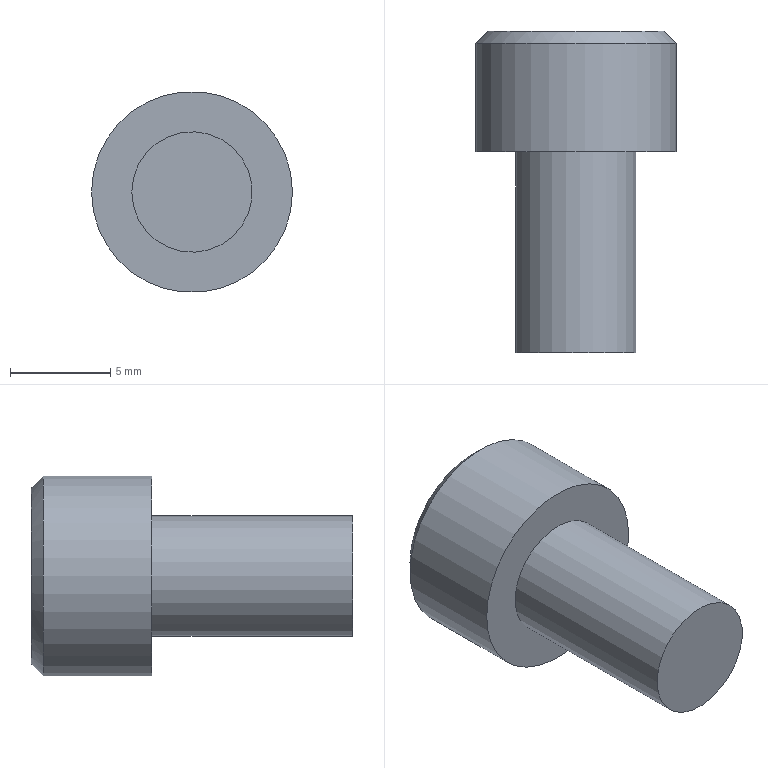Part | NX | features 5003_326_CB6-10 2 | 1 solid | 19 faces | box 10 x 16 x 10 mm | volume 673.77 mm3 | plane 15 | cylinder 2 | cone 2 | commonest cylinder face diameters 6 x1 10 x1
STEP:
#1=CARTESIAN_POINT('',(170.225,6.,-39.5));
#2=VERTEX_POINT('',#1);
#3=CARTESIAN_POINT('',(165.825,6.,-39.5));
#4=DIRECTION('',(0.,-1.,0.));
#5=DIRECTION('',(1.,0.,0.));
#6=AXIS2_PLACEMENT_3D('',#3,#4,#5);
#7=CIRCLE('',#6,4.4);
#8=EDGE_CURVE('',#2,#2,#7,.F.);
#9=ORIENTED_EDGE('',*,*,#8,.T.);
#10=EDGE_LOOP('',(#9));
#11=FACE_BOUND('',#10,.T.);
#12=CARTESIAN_POINT('',(165.825,6.,-42.387));
#13=VERTEX_POINT('',#12);
#14=CARTESIAN_POINT('',(163.325,6.,-40.943));
#15=VERTEX_POINT('',#14);
#16=CARTESIAN_POINT('',(165.825,6.,-42.387));
#17=DIRECTION('',(-0.866,0.,0.5));
#18=VECTOR('',#17,1000.);
#19=LINE('',#16,#18);
#20=EDGE_CURVE('',#13,#15,#19,.T.);
#21=ORIENTED_EDGE('',*,*,#20,.F.);
#22=CARTESIAN_POINT('',(168.325,6.,-40.943));
#23=VERTEX_POINT('',#22);
#24=CARTESIAN_POINT('',(168.325,6.,-40.943));
#25=DIRECTION('',(-0.866,0.,-0.5));
#26=VECTOR('',#25,1000.);
#27=LINE('',#24,#26);
#28=EDGE_CURVE('',#23,#13,#27,.T.);
#29=ORIENTED_EDGE('',*,*,#28,.F.);
#30=CARTESIAN_POINT('',(168.325,6.,-38.057));
#31=VERTEX_POINT('',#30);
#32=CARTESIAN_POINT('',(168.325,6.,-38.057));
#33=DIRECTION('',(0.,0.,-1.));
#34=VECTOR('',#33,1000.);
#35=LINE('',#32,#34);
#36=EDGE_CURVE('',#31,#23,#35,.T.);
#37=ORIENTED_EDGE('',*,*,#36,.F.);
#38=CARTESIAN_POINT('',(165.825,6.,-36.613));
#39=VERTEX_POINT('',#38);
#40=CARTESIAN_POINT('',(165.825,6.,-36.613));
#41=DIRECTION('',(0.866,0.,-0.5));
#42=VECTOR('',#41,1000.);
#43=LINE('',#40,#42);
#44=EDGE_CURVE('',#39,#31,#43,.T.);
#45=ORIENTED_EDGE('',*,*,#44,.F.);
#46=CARTESIAN_POINT('',(163.325,6.,-38.057));
#47=VERTEX_POINT('',#46);
#48=CARTESIAN_POINT('',(163.325,6.,-38.057));
#49=DIRECTION('',(0.866,0.,0.5));
#50=VECTOR('',#49,1000.);
#51=LINE('',#48,#50);
#52=EDGE_CURVE('',#47,#39,#51,.T.);
#53=ORIENTED_EDGE('',*,*,#52,.F.);
#54=CARTESIAN_POINT('',(163.325,6.,-40.943));
#55=DIRECTION('',(0.,0.,1.));
#56=VECTOR('',#55,1000.);
#57=LINE('',#54,#56);
#58=EDGE_CURVE('',#15,#47,#57,.T.);
#59=ORIENTED_EDGE('',*,*,#58,.F.);
#60=EDGE_LOOP('',(#21,#29,#37,#45,#53,#59));
#61=FACE_BOUND('',#60,.T.);
#62=CARTESIAN_POINT('',(165.825,6.,-34.5));
#63=DIRECTION('',(0.,-1.,0.));
#64=DIRECTION('',(1.,0.,0.));
#65=AXIS2_PLACEMENT_3D('',#62,#63,#64);
#66=PLANE('',#65);
#67=ADVANCED_FACE('',(#11,#61),#66,.F.);
#68=CARTESIAN_POINT('',(162.825,-10.,-39.5));
#69=VERTEX_POINT('',#68);
#70=CARTESIAN_POINT('',(165.825,-10.,-39.5));
#71=DIRECTION('',(0.,1.,0.));
#72=DIRECTION('',(-1.,0.,0.));
#73=AXIS2_PLACEMENT_3D('',#70,#71,#72);
#74=CIRCLE('',#73,3.);
#75=EDGE_CURVE('',#69,#69,#74,.T.);
#76=ORIENTED_EDGE('',*,*,#75,.F.);
#77=EDGE_LOOP('',(#76));
#78=FACE_BOUND('',#77,.T.);
#79=CARTESIAN_POINT('',(165.825,-10.,-39.5));
#80=DIRECTION('',(0.,1.,0.));
#81=DIRECTION('',(-1.,0.,0.));
#82=AXIS2_PLACEMENT_3D('',#79,#80,#81);
#83=PLANE('',#82);
#84=ADVANCED_FACE('',(#78),#83,.F.);
#85=CARTESIAN_POINT('',(162.825,0.,-39.5));
#86=VERTEX_POINT('',#85);
#87=CARTESIAN_POINT('',(165.825,0.,-39.5));
#88=DIRECTION('',(0.,1.,0.));
#89=DIRECTION('',(-1.,0.,0.));
#90=AXIS2_PLACEMENT_3D('',#87,#88,#89);
#91=CIRCLE('',#90,3.);
#92=EDGE_CURVE('',#86,#86,#91,.T.);
#93=ORIENTED_EDGE('',*,*,#92,.F.);
#94=EDGE_LOOP('',(#93));
#95=FACE_BOUND('',#94,.T.);
#96=ORIENTED_EDGE('',*,*,#75,.T.);
#97=EDGE_LOOP('',(#96));
#98=FACE_BOUND('',#97,.T.);
#99=CARTESIAN_POINT('',(165.825,6.,-39.5));
#100=DIRECTION('',(0.,1.,0.));
#101=DIRECTION('',(-1.,0.,0.));
#102=AXIS2_PLACEMENT_3D('',#99,#100,#101);
#103=CYLINDRICAL_SURFACE('',#102,3.);
#104=ADVANCED_FACE('',(#95,#98),#103,.T.);
#105=CARTESIAN_POINT('',(160.825,0.,-39.5));
#106=VERTEX_POINT('',#105);
#107=CARTESIAN_POINT('',(165.825,0.,-39.5));
#108=DIRECTION('',(0.,1.,0.));
#109=DIRECTION('',(-1.,0.,0.));
#110=AXIS2_PLACEMENT_3D('',#107,#108,#109);
#111=CIRCLE('',#110,5.);
#112=EDGE_CURVE('',#106,#106,#111,.T.);
#113=ORIENTED_EDGE('',*,*,#112,.F.);
#114=EDGE_LOOP('',(#113));
#115=FACE_BOUND('',#114,.T.);
#116=ORIENTED_EDGE('',*,*,#92,.T.);
#117=EDGE_LOOP('',(#116));
#118=FACE_BOUND('',#117,.T.);
#119=CARTESIAN_POINT('',(165.825,0.,-36.5));
#120=DIRECTION('',(0.,1.,0.));
#121=DIRECTION('',(-1.,0.,0.));
#122=AXIS2_PLACEMENT_3D('',#119,#120,#121);
#123=PLANE('',#122);
#124=ADVANCED_FACE('',(#115,#118),#123,.F.);
#125=CARTESIAN_POINT('',(170.825,5.4,-39.5));
#126=VERTEX_POINT('',#125);
#127=CARTESIAN_POINT('',(165.825,5.4,-39.5));
#128=DIRECTION('',(0.,-1.,0.));
#129=DIRECTION('',(1.,0.,0.));
#130=AXIS2_PLACEMENT_3D('',#127,#128,#129);
#131=CIRCLE('',#130,5.);
#132=EDGE_CURVE('',#126,#126,#131,.T.);
#133=ORIENTED_EDGE('',*,*,#132,.T.);
#134=EDGE_LOOP('',(#133));
#135=FACE_BOUND('',#134,.T.);
#136=ORIENTED_EDGE('',*,*,#112,.T.);
#137=EDGE_LOOP('',(#136));
#138=FACE_BOUND('',#137,.T.);
#139=CARTESIAN_POINT('',(165.825,6.,-39.5));
#140=DIRECTION('',(0.,1.,0.));
#141=DIRECTION('',(-1.,0.,0.));
#142=AXIS2_PLACEMENT_3D('',#139,#140,#141);
#143=CYLINDRICAL_SURFACE('',#142,5.);
#144=ADVANCED_FACE('',(#135,#138),#143,.T.);
#145=ORIENTED_EDGE('',*,*,#132,.F.);
#146=EDGE_LOOP('',(#145));
#147=FACE_BOUND('',#146,.T.);
#148=ORIENTED_EDGE('',*,*,#8,.F.);
#149=EDGE_LOOP('',(#148));
#150=FACE_BOUND('',#149,.T.);
#151=CARTESIAN_POINT('',(165.825,6.,-39.5));
#152=DIRECTION('',(0.,-1.,0.));
#153=DIRECTION('',(1.,0.,0.));
#154=AXIS2_PLACEMENT_3D('',#151,#152,#153);
#155=CONICAL_SURFACE('',#154,4.4,0.7854);
#156=ADVANCED_FACE('',(#147,#150),#155,.T.);
#157=CARTESIAN_POINT('',(168.325,3.,-40.943));
#158=VERTEX_POINT('',#157);
#159=CARTESIAN_POINT('',(167.075,3.,-41.665));
#160=VERTEX_POINT('',#159);
#161=CARTESIAN_POINT('',(168.325,3.,-40.943));
#162=DIRECTION('',(-0.866,0.,-0.5));
#163=VECTOR('',#162,1000.);
#164=LINE('',#161,#163);
#165=EDGE_CURVE('',#158,#160,#164,.T.);
#166=ORIENTED_EDGE('',*,*,#165,.F.);
#167=CARTESIAN_POINT('',(168.325,3.,-40.943));
#168=DIRECTION('',(0.,1.,0.));
#169=VECTOR('',#168,1000.);
#170=LINE('',#167,#169);
#171=EDGE_CURVE('',#158,#23,#170,.T.);
#172=ORIENTED_EDGE('',*,*,#171,.T.);
#173=ORIENTED_EDGE('',*,*,#28,.T.);
#174=CARTESIAN_POINT('',(165.825,3.,-42.387));
#175=VERTEX_POINT('',#174);
#176=CARTESIAN_POINT('',(165.825,3.,-42.387));
#177=DIRECTION('',(0.,1.,0.));
#178=VECTOR('',#177,1000.);
#179=LINE('',#176,#178);
#180=EDGE_CURVE('',#175,#13,#179,.T.);
#181=ORIENTED_EDGE('',*,*,#180,.F.);
#182=CARTESIAN_POINT('',(168.325,3.,-40.943));
#183=DIRECTION('',(-0.866,0.,-0.5));
#184=VECTOR('',#183,1000.);
#185=LINE('',#182,#184);
#186=EDGE_CURVE('',#160,#175,#185,.T.);
#187=ORIENTED_EDGE('',*,*,#186,.F.);
#188=EDGE_LOOP('',(#166,#172,#173,#181,#187));
#189=FACE_BOUND('',#188,.T.);
#190=CARTESIAN_POINT('',(168.325,3.,-40.943));
#191=DIRECTION('',(0.5,0.,-0.866));
#192=DIRECTION('',(0.866,0.,0.5));
#193=AXIS2_PLACEMENT_3D('',#190,#191,#192);
#194=PLANE('',#193);
#195=ADVANCED_FACE('',(#189),#194,.F.);
#196=CARTESIAN_POINT('',(168.325,3.,-38.057));
#197=VERTEX_POINT('',#196);
#198=CARTESIAN_POINT('',(168.325,3.,-39.5));
#199=VERTEX_POINT('',#198);
#200=CARTESIAN_POINT('',(168.325,3.,-38.057));
#201=DIRECTION('',(0.,0.,-1.));
#202=VECTOR('',#201,1000.);
#203=LINE('',#200,#202);
#204=EDGE_CURVE('',#197,#199,#203,.T.);
#205=ORIENTED_EDGE('',*,*,#204,.F.);
#206=CARTESIAN_POINT('',(168.325,3.,-38.057));
#207=DIRECTION('',(0.,1.,0.));
#208=VECTOR('',#207,1000.);
#209=LINE('',#206,#208);
#210=EDGE_CURVE('',#197,#31,#209,.T.);
#211=ORIENTED_EDGE('',*,*,#210,.T.);
#212=ORIENTED_EDGE('',*,*,#36,.T.);
#213=ORIENTED_EDGE('',*,*,#171,.F.);
#214=CARTESIAN_POINT('',(168.325,3.,-38.057));
#215=DIRECTION('',(0.,0.,-1.));
#216=VECTOR('',#215,1000.);
#217=LINE('',#214,#216);
#218=EDGE_CURVE('',#199,#158,#217,.T.);
#219=ORIENTED_EDGE('',*,*,#218,.F.);
#220=EDGE_LOOP('',(#205,#211,#212,#213,#219));
#221=FACE_BOUND('',#220,.T.);
#222=CARTESIAN_POINT('',(168.325,3.,-38.057));
#223=DIRECTION('',(1.,0.,0.));
#224=DIRECTION('',(0.,0.,1.));
#225=AXIS2_PLACEMENT_3D('',#222,#223,#224);
#226=PLANE('',#225);
#227=ADVANCED_FACE('',(#221),#226,.F.);
#228=CARTESIAN_POINT('',(165.825,3.,-36.613));
#229=VERTEX_POINT('',#228);
#230=CARTESIAN_POINT('',(167.075,3.,-37.335));
#231=VERTEX_POINT('',#230);
#232=CARTESIAN_POINT('',(165.825,3.,-36.613));
#233=DIRECTION('',(0.866,0.,-0.5));
#234=VECTOR('',#233,1000.);
#235=LINE('',#232,#234);
#236=EDGE_CURVE('',#229,#231,#235,.T.);
#237=ORIENTED_EDGE('',*,*,#236,.F.);
#238=CARTESIAN_POINT('',(165.825,3.,-36.613));
#239=DIRECTION('',(0.,1.,0.));
#240=VECTOR('',#239,1000.);
#241=LINE('',#238,#240);
#242=EDGE_CURVE('',#229,#39,#241,.T.);
#243=ORIENTED_EDGE('',*,*,#242,.T.);
#244=ORIENTED_EDGE('',*,*,#44,.T.);
#245=ORIENTED_EDGE('',*,*,#210,.F.);
#246=CARTESIAN_POINT('',(165.825,3.,-36.613));
#247=DIRECTION('',(0.866,0.,-0.5));
#248=VECTOR('',#247,1000.);
#249=LINE('',#246,#248);
#250=EDGE_CURVE('',#231,#197,#249,.T.);
#251=ORIENTED_EDGE('',*,*,#250,.F.);
#252=EDGE_LOOP('',(#237,#243,#244,#245,#251));
#253=FACE_BOUND('',#252,.T.);
#254=CARTESIAN_POINT('',(165.825,3.,-36.613));
#255=DIRECTION('',(0.5,0.,0.866));
#256=DIRECTION('',(-0.866,0.,0.5));
#257=AXIS2_PLACEMENT_3D('',#254,#255,#256);
#258=PLANE('',#257);
#259=ADVANCED_FACE('',(#253),#258,.F.);
#260=CARTESIAN_POINT('',(163.325,3.,-38.057));
#261=VERTEX_POINT('',#260);
#262=CARTESIAN_POINT('',(164.575,3.,-37.335));
#263=VERTEX_POINT('',#262);
#264=CARTESIAN_POINT('',(163.325,3.,-38.057));
#265=DIRECTION('',(0.866,0.,0.5));
#266=VECTOR('',#265,1000.);
#267=LINE('',#264,#266);
#268=EDGE_CURVE('',#261,#263,#267,.T.);
#269=ORIENTED_EDGE('',*,*,#268,.F.);
#270=CARTESIAN_POINT('',(163.325,3.,-38.057));
#271=DIRECTION('',(0.,1.,0.));
#272=VECTOR('',#271,1000.);
#273=LINE('',#270,#272);
#274=EDGE_CURVE('',#261,#47,#273,.T.);
#275=ORIENTED_EDGE('',*,*,#274,.T.);
#276=ORIENTED_EDGE('',*,*,#52,.T.);
#277=ORIENTED_EDGE('',*,*,#242,.F.);
#278=CARTESIAN_POINT('',(163.325,3.,-38.057));
#279=DIRECTION('',(0.866,0.,0.5));
#280=VECTOR('',#279,1000.);
#281=LINE('',#278,#280);
#282=EDGE_CURVE('',#263,#229,#281,.T.);
#283=ORIENTED_EDGE('',*,*,#282,.F.);
#284=EDGE_LOOP('',(#269,#275,#276,#277,#283));
#285=FACE_BOUND('',#284,.T.);
#286=CARTESIAN_POINT('',(163.325,3.,-38.057));
#287=DIRECTION('',(-0.5,0.,0.866));
#288=DIRECTION('',(-0.866,0.,-0.5));
#289=AXIS2_PLACEMENT_3D('',#286,#287,#288);
#290=PLANE('',#289);
#291=ADVANCED_FACE('',(#285),#290,.F.);
#292=CARTESIAN_POINT('',(163.325,3.,-40.943));
#293=VERTEX_POINT('',#292);
#294=CARTESIAN_POINT('',(163.325,3.,-39.5));
#295=VERTEX_POINT('',#294);
#296=CARTESIAN_POINT('',(163.325,3.,-40.943));
#297=DIRECTION('',(0.,0.,1.));
#298=VECTOR('',#297,1000.);
#299=LINE('',#296,#298);
#300=EDGE_CURVE('',#293,#295,#299,.T.);
#301=ORIENTED_EDGE('',*,*,#300,.F.);
#302=CARTESIAN_POINT('',(163.325,3.,-40.943));
#303=DIRECTION('',(0.,1.,0.));
#304=VECTOR('',#303,1000.);
#305=LINE('',#302,#304);
#306=EDGE_CURVE('',#293,#15,#305,.T.);
#307=ORIENTED_EDGE('',*,*,#306,.T.);
#308=ORIENTED_EDGE('',*,*,#58,.T.);
#309=ORIENTED_EDGE('',*,*,#274,.F.);
#310=CARTESIAN_POINT('',(163.325,3.,-40.943));
#311=DIRECTION('',(0.,0.,1.));
#312=VECTOR('',#311,1000.);
#313=LINE('',#310,#312);
#314=EDGE_CURVE('',#295,#261,#313,.T.);
#315=ORIENTED_EDGE('',*,*,#314,.F.);
#316=EDGE_LOOP('',(#301,#307,#308,#309,#315));
#317=FACE_BOUND('',#316,.T.);
#318=CARTESIAN_POINT('',(163.325,3.,-40.943));
#319=DIRECTION('',(-1.,0.,0.));
#320=DIRECTION('',(0.,-1.,0.));
#321=AXIS2_PLACEMENT_3D('',#318,#319,#320);
#322=PLANE('',#321);
#323=ADVANCED_FACE('',(#317),#322,.F.);
#324=CARTESIAN_POINT('',(164.575,3.,-41.665));
#325=VERTEX_POINT('',#324);
#326=CARTESIAN_POINT('',(165.825,3.,-42.387));
#327=DIRECTION('',(-0.866,0.,0.5));
#328=VECTOR('',#327,1000.);
#329=LINE('',#326,#328);
#330=EDGE_CURVE('',#175,#325,#329,.T.);
#331=ORIENTED_EDGE('',*,*,#330,.F.);
#332=ORIENTED_EDGE('',*,*,#180,.T.);
#333=ORIENTED_EDGE('',*,*,#20,.T.);
#334=ORIENTED_EDGE('',*,*,#306,.F.);
#335=CARTESIAN_POINT('',(165.825,3.,-42.387));
#336=DIRECTION('',(-0.866,0.,0.5));
#337=VECTOR('',#336,1000.);
#338=LINE('',#335,#337);
#339=EDGE_CURVE('',#325,#293,#338,.T.);
#340=ORIENTED_EDGE('',*,*,#339,.F.);
#341=EDGE_LOOP('',(#331,#332,#333,#334,#340));
#342=FACE_BOUND('',#341,.T.);
#343=CARTESIAN_POINT('',(165.825,3.,-42.387));
#344=DIRECTION('',(-0.5,0.,-0.866));
#345=DIRECTION('',(0.866,0.,-0.5));
#346=AXIS2_PLACEMENT_3D('',#343,#344,#345);
#347=PLANE('',#346);
#348=ADVANCED_FACE('',(#342),#347,.F.);
#349=ORIENTED_EDGE('',*,*,#314,.T.);
#350=ORIENTED_EDGE('',*,*,#268,.T.);
#351=CARTESIAN_POINT('',(165.825,3.,-39.5));
#352=DIRECTION('',(0.,1.,0.));
#353=DIRECTION('',(0.,0.,-1.));
#354=AXIS2_PLACEMENT_3D('',#351,#352,#353);
#355=CIRCLE('',#354,2.5);
#356=EDGE_CURVE('',#295,#263,#355,.T.);
#357=ORIENTED_EDGE('',*,*,#356,.F.);
#358=EDGE_LOOP('',(#349,#350,#357));
#359=FACE_BOUND('',#358,.T.);
#360=CARTESIAN_POINT('',(165.825,3.,-39.5));
#361=DIRECTION('',(0.,1.,0.));
#362=DIRECTION('',(-1.,0.,0.));
#363=AXIS2_PLACEMENT_3D('',#360,#361,#362);
#364=PLANE('',#363);
#365=ADVANCED_FACE('',(#359),#364,.T.);
#366=ORIENTED_EDGE('',*,*,#282,.T.);
#367=ORIENTED_EDGE('',*,*,#236,.T.);
#368=CARTESIAN_POINT('',(165.825,3.,-39.5));
#369=DIRECTION('',(0.,1.,0.));
#370=DIRECTION('',(0.,0.,-1.));
#371=AXIS2_PLACEMENT_3D('',#368,#369,#370);
#372=CIRCLE('',#371,2.5);
#373=EDGE_CURVE('',#263,#231,#372,.T.);
#374=ORIENTED_EDGE('',*,*,#373,.F.);
#375=EDGE_LOOP('',(#366,#367,#374));
#376=FACE_BOUND('',#375,.T.);
#377=CARTESIAN_POINT('',(165.825,3.,-39.5));
#378=DIRECTION('',(0.,1.,0.));
#379=DIRECTION('',(-1.,0.,0.));
#380=AXIS2_PLACEMENT_3D('',#377,#378,#379);
#381=PLANE('',#380);
#382=ADVANCED_FACE('',(#376),#381,.T.);
#383=ORIENTED_EDGE('',*,*,#250,.T.);
#384=ORIENTED_EDGE('',*,*,#204,.T.);
#385=CARTESIAN_POINT('',(165.825,3.,-39.5));
#386=DIRECTION('',(0.,1.,0.));
#387=DIRECTION('',(0.,0.,-1.));
#388=AXIS2_PLACEMENT_3D('',#385,#386,#387);
#389=CIRCLE('',#388,2.5);
#390=EDGE_CURVE('',#231,#199,#389,.T.);
#391=ORIENTED_EDGE('',*,*,#390,.F.);
#392=EDGE_LOOP('',(#383,#384,#391));
#393=FACE_BOUND('',#392,.T.);
#394=CARTESIAN_POINT('',(165.825,3.,-39.5));
#395=DIRECTION('',(0.,1.,0.));
#396=DIRECTION('',(-1.,0.,0.));
#397=AXIS2_PLACEMENT_3D('',#394,#395,#396);
#398=PLANE('',#397);
#399=ADVANCED_FACE('',(#393),#398,.T.);
#400=ORIENTED_EDGE('',*,*,#218,.T.);
#401=ORIENTED_EDGE('',*,*,#165,.T.);
#402=CARTESIAN_POINT('',(165.825,3.,-39.5));
#403=DIRECTION('',(0.,1.,0.));
#404=DIRECTION('',(0.,0.,-1.));
#405=AXIS2_PLACEMENT_3D('',#402,#403,#404);
#406=CIRCLE('',#405,2.5);
#407=EDGE_CURVE('',#199,#160,#406,.T.);
#408=ORIENTED_EDGE('',*,*,#407,.F.);
#409=EDGE_LOOP('',(#400,#401,#408));
#410=FACE_BOUND('',#409,.T.);
#411=CARTESIAN_POINT('',(165.825,3.,-39.5));
#412=DIRECTION('',(0.,1.,0.));
#413=DIRECTION('',(-1.,0.,0.));
#414=AXIS2_PLACEMENT_3D('',#411,#412,#413);
#415=PLANE('',#414);
#416=ADVANCED_FACE('',(#410),#415,.T.);
#417=ORIENTED_EDGE('',*,*,#186,.T.);
#418=ORIENTED_EDGE('',*,*,#330,.T.);
#419=CARTESIAN_POINT('',(165.825,3.,-39.5));
#420=DIRECTION('',(0.,1.,0.));
#421=DIRECTION('',(0.,0.,-1.));
#422=AXIS2_PLACEMENT_3D('',#419,#420,#421);
#423=CIRCLE('',#422,2.5);
#424=EDGE_CURVE('',#160,#325,#423,.T.);
#425=ORIENTED_EDGE('',*,*,#424,.F.);
#426=EDGE_LOOP('',(#417,#418,#425));
#427=FACE_BOUND('',#426,.T.);
#428=CARTESIAN_POINT('',(165.825,3.,-39.5));
#429=DIRECTION('',(0.,1.,0.));
#430=DIRECTION('',(-1.,0.,0.));
#431=AXIS2_PLACEMENT_3D('',#428,#429,#430);
#432=PLANE('',#431);
#433=ADVANCED_FACE('',(#427),#432,.T.);
#434=ORIENTED_EDGE('',*,*,#339,.T.);
#435=ORIENTED_EDGE('',*,*,#300,.T.);
#436=CARTESIAN_POINT('',(165.825,3.,-39.5));
#437=DIRECTION('',(0.,1.,0.));
#438=DIRECTION('',(0.,0.,-1.));
#439=AXIS2_PLACEMENT_3D('',#436,#437,#438);
#440=CIRCLE('',#439,2.5);
#441=EDGE_CURVE('',#325,#295,#440,.T.);
#442=ORIENTED_EDGE('',*,*,#441,.F.);
#443=EDGE_LOOP('',(#434,#435,#442));
#444=FACE_BOUND('',#443,.T.);
#445=CARTESIAN_POINT('',(165.825,3.,-39.5));
#446=DIRECTION('',(0.,1.,0.));
#447=DIRECTION('',(-1.,0.,0.));
#448=AXIS2_PLACEMENT_3D('',#445,#446,#447);
#449=PLANE('',#448);
#450=ADVANCED_FACE('',(#444),#449,.T.);
#451=ORIENTED_EDGE('',*,*,#441,.T.);
#452=ORIENTED_EDGE('',*,*,#356,.T.);
#453=ORIENTED_EDGE('',*,*,#373,.T.);
#454=ORIENTED_EDGE('',*,*,#390,.T.);
#455=ORIENTED_EDGE('',*,*,#407,.T.);
#456=ORIENTED_EDGE('',*,*,#424,.T.);
#457=EDGE_LOOP('',(#451,#452,#453,#454,#455,#456));
#458=FACE_BOUND('',#457,.T.);
#459=CARTESIAN_POINT('',(165.825,1.498,-39.5));
#460=VERTEX_POINT('',#459);
#461=VERTEX_LOOP('',#460);
#462=FACE_BOUND('',#461,.T.);
#463=CARTESIAN_POINT('',(165.825,1.498,-39.5));
#464=DIRECTION('',(0.,1.,0.));
#465=DIRECTION('',(0.,0.,-1.));
#466=AXIS2_PLACEMENT_3D('',#463,#464,#465);
#467=CONICAL_SURFACE('',#466,0.,1.03);
#468=ADVANCED_FACE('',(#458,#462),#467,.F.);
#469=CLOSED_SHELL('',(#67,#84,#104,#124,#144,#156,#195,#227,#259,#291,#323,#348,#365,#382,#399,#416,#433,#450,#468));
#470=MANIFOLD_SOLID_BREP('',#469);
#471=(LENGTH_UNIT()NAMED_UNIT(*)SI_UNIT(.MILLI.,.METRE.));
#472=UNCERTAINTY_MEASURE_WITH_UNIT(LENGTH_MEASURE(0.00001),#471,'','');
#473=(NAMED_UNIT(*)PLANE_ANGLE_UNIT()SI_UNIT($,.RADIAN.));
#474=(NAMED_UNIT(*)SI_UNIT($,.STERADIAN.)SOLID_ANGLE_UNIT());
#475=(GEOMETRIC_REPRESENTATION_CONTEXT(3)GLOBAL_UNCERTAINTY_ASSIGNED_CONTEXT((#472))GLOBAL_UNIT_ASSIGNED_CONTEXT((#471,#473,#474))REPRESENTATION_CONTEXT('',''));
#476=ADVANCED_BREP_SHAPE_REPRESENTATION('',(#470),#475);